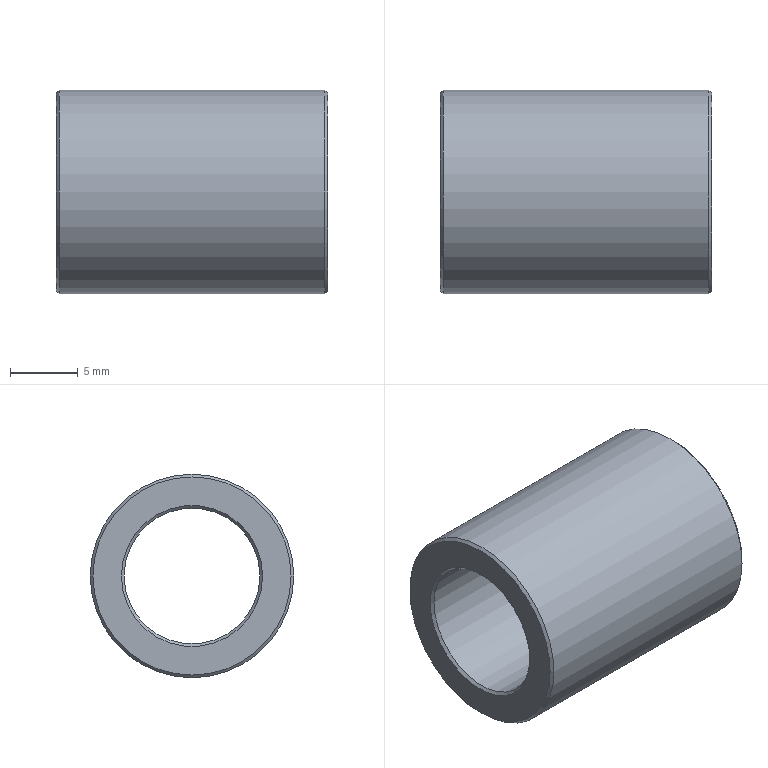Part | NX | features 5003_024_C-KNCLA10-15-20 2 | 1 solid | 8 faces | box 20 x 15 x 15 mm | volume 1960 mm3 | cone 4 | plane 2 | cylinder 2 | commonest cylinder face diameters 10 x1 15 x1
STEP:
#1=CARTESIAN_POINT('',(-233.475,-518.7,-147.));
#2=VERTEX_POINT('',#1);
#3=CARTESIAN_POINT('',(-233.475,-526.,-147.));
#4=DIRECTION('',(1.,0.,0.));
#5=DIRECTION('',(0.,1.,0.));
#6=AXIS2_PLACEMENT_3D('',#3,#4,#5);
#7=CIRCLE('',#6,7.3);
#8=EDGE_CURVE('',#2,#2,#7,.F.);
#9=ORIENTED_EDGE('',*,*,#8,.T.);
#10=EDGE_LOOP('',(#9));
#11=FACE_BOUND('',#10,.T.);
#12=CARTESIAN_POINT('',(-233.475,-520.8,-147.));
#13=VERTEX_POINT('',#12);
#14=CARTESIAN_POINT('',(-233.475,-526.,-147.));
#15=DIRECTION('',(1.,0.,0.));
#16=DIRECTION('',(0.,1.,0.));
#17=AXIS2_PLACEMENT_3D('',#14,#15,#16);
#18=CIRCLE('',#17,5.2);
#19=EDGE_CURVE('',#13,#13,#18,.T.);
#20=ORIENTED_EDGE('',*,*,#19,.T.);
#21=EDGE_LOOP('',(#20));
#22=FACE_BOUND('',#21,.T.);
#23=CARTESIAN_POINT('',(-233.475,-521.,-147.));
#24=DIRECTION('',(1.,0.,0.));
#25=DIRECTION('',(0.,1.,0.));
#26=AXIS2_PLACEMENT_3D('',#23,#24,#25);
#27=PLANE('',#26);
#28=ADVANCED_FACE('',(#11,#22),#27,.F.);
#29=CARTESIAN_POINT('',(-213.675,-533.5,-147.));
#30=VERTEX_POINT('',#29);
#31=CARTESIAN_POINT('',(-213.675,-526.,-147.));
#32=DIRECTION('',(-1.,0.,0.));
#33=DIRECTION('',(0.,-1.,0.));
#34=AXIS2_PLACEMENT_3D('',#31,#32,#33);
#35=CIRCLE('',#34,7.5);
#36=EDGE_CURVE('',#30,#30,#35,.T.);
#37=ORIENTED_EDGE('',*,*,#36,.T.);
#38=EDGE_LOOP('',(#37));
#39=FACE_BOUND('',#38,.T.);
#40=CARTESIAN_POINT('',(-233.275,-518.5,-147.));
#41=VERTEX_POINT('',#40);
#42=CARTESIAN_POINT('',(-233.275,-526.,-147.));
#43=DIRECTION('',(1.,0.,0.));
#44=DIRECTION('',(0.,1.,0.));
#45=AXIS2_PLACEMENT_3D('',#42,#43,#44);
#46=CIRCLE('',#45,7.5);
#47=EDGE_CURVE('',#41,#41,#46,.T.);
#48=ORIENTED_EDGE('',*,*,#47,.T.);
#49=EDGE_LOOP('',(#48));
#50=FACE_BOUND('',#49,.T.);
#51=CARTESIAN_POINT('',(-237.616,-526.,-147.));
#52=DIRECTION('',(-1.,0.,0.));
#53=DIRECTION('',(0.,-1.,0.));
#54=AXIS2_PLACEMENT_3D('',#51,#52,#53);
#55=CYLINDRICAL_SURFACE('',#54,7.5);
#56=ADVANCED_FACE('',(#39,#50),#55,.T.);
#57=CARTESIAN_POINT('',(-213.475,-533.3,-147.));
#58=VERTEX_POINT('',#57);
#59=CARTESIAN_POINT('',(-213.475,-526.,-147.));
#60=DIRECTION('',(-1.,0.,0.));
#61=DIRECTION('',(0.,-1.,0.));
#62=AXIS2_PLACEMENT_3D('',#59,#60,#61);
#63=CIRCLE('',#62,7.3);
#64=EDGE_CURVE('',#58,#58,#63,.F.);
#65=ORIENTED_EDGE('',*,*,#64,.T.);
#66=EDGE_LOOP('',(#65));
#67=FACE_BOUND('',#66,.T.);
#68=CARTESIAN_POINT('',(-213.475,-531.2,-147.));
#69=VERTEX_POINT('',#68);
#70=CARTESIAN_POINT('',(-213.475,-526.,-147.));
#71=DIRECTION('',(-1.,0.,0.));
#72=DIRECTION('',(0.,-1.,0.));
#73=AXIS2_PLACEMENT_3D('',#70,#71,#72);
#74=CIRCLE('',#73,5.2);
#75=EDGE_CURVE('',#69,#69,#74,.T.);
#76=ORIENTED_EDGE('',*,*,#75,.T.);
#77=EDGE_LOOP('',(#76));
#78=FACE_BOUND('',#77,.T.);
#79=CARTESIAN_POINT('',(-213.475,-521.,-147.));
#80=DIRECTION('',(-1.,0.,0.));
#81=DIRECTION('',(0.,-1.,0.));
#82=AXIS2_PLACEMENT_3D('',#79,#80,#81);
#83=PLANE('',#82);
#84=ADVANCED_FACE('',(#67,#78),#83,.F.);
#85=CARTESIAN_POINT('',(-213.675,-531.,-147.));
#86=VERTEX_POINT('',#85);
#87=CARTESIAN_POINT('',(-213.675,-526.,-147.));
#88=DIRECTION('',(-1.,0.,0.));
#89=DIRECTION('',(0.,-1.,0.));
#90=AXIS2_PLACEMENT_3D('',#87,#88,#89);
#91=CIRCLE('',#90,5.);
#92=EDGE_CURVE('',#86,#86,#91,.F.);
#93=ORIENTED_EDGE('',*,*,#92,.T.);
#94=EDGE_LOOP('',(#93));
#95=FACE_BOUND('',#94,.T.);
#96=CARTESIAN_POINT('',(-233.275,-521.,-147.));
#97=VERTEX_POINT('',#96);
#98=CARTESIAN_POINT('',(-233.275,-526.,-147.));
#99=DIRECTION('',(1.,0.,0.));
#100=DIRECTION('',(0.,1.,0.));
#101=AXIS2_PLACEMENT_3D('',#98,#99,#100);
#102=CIRCLE('',#101,5.);
#103=EDGE_CURVE('',#97,#97,#102,.F.);
#104=ORIENTED_EDGE('',*,*,#103,.T.);
#105=EDGE_LOOP('',(#104));
#106=FACE_BOUND('',#105,.T.);
#107=CARTESIAN_POINT('',(-237.616,-526.,-147.));
#108=DIRECTION('',(-1.,0.,0.));
#109=DIRECTION('',(0.,-1.,0.));
#110=AXIS2_PLACEMENT_3D('',#107,#108,#109);
#111=CYLINDRICAL_SURFACE('',#110,5.);
#112=ADVANCED_FACE('',(#95,#106),#111,.F.);
#113=ORIENTED_EDGE('',*,*,#64,.F.);
#114=EDGE_LOOP('',(#113));
#115=FACE_BOUND('',#114,.T.);
#116=ORIENTED_EDGE('',*,*,#36,.F.);
#117=EDGE_LOOP('',(#116));
#118=FACE_BOUND('',#117,.T.);
#119=CARTESIAN_POINT('',(-213.675,-526.,-147.));
#120=DIRECTION('',(-1.,0.,0.));
#121=DIRECTION('',(0.,-1.,0.));
#122=AXIS2_PLACEMENT_3D('',#119,#120,#121);
#123=CONICAL_SURFACE('',#122,7.5,0.7854);
#124=ADVANCED_FACE('',(#115,#118),#123,.T.);
#125=ORIENTED_EDGE('',*,*,#92,.F.);
#126=EDGE_LOOP('',(#125));
#127=FACE_BOUND('',#126,.T.);
#128=ORIENTED_EDGE('',*,*,#75,.F.);
#129=EDGE_LOOP('',(#128));
#130=FACE_BOUND('',#129,.T.);
#131=CARTESIAN_POINT('',(-213.475,-526.,-147.));
#132=DIRECTION('',(1.,0.,0.));
#133=DIRECTION('',(0.,1.,0.));
#134=AXIS2_PLACEMENT_3D('',#131,#132,#133);
#135=CONICAL_SURFACE('',#134,5.2,0.7854);
#136=ADVANCED_FACE('',(#127,#130),#135,.F.);
#137=ORIENTED_EDGE('',*,*,#47,.F.);
#138=EDGE_LOOP('',(#137));
#139=FACE_BOUND('',#138,.T.);
#140=ORIENTED_EDGE('',*,*,#8,.F.);
#141=EDGE_LOOP('',(#140));
#142=FACE_BOUND('',#141,.T.);
#143=CARTESIAN_POINT('',(-233.475,-526.,-147.));
#144=DIRECTION('',(1.,0.,0.));
#145=DIRECTION('',(0.,1.,0.));
#146=AXIS2_PLACEMENT_3D('',#143,#144,#145);
#147=CONICAL_SURFACE('',#146,7.3,0.7854);
#148=ADVANCED_FACE('',(#139,#142),#147,.T.);
#149=ORIENTED_EDGE('',*,*,#19,.F.);
#150=EDGE_LOOP('',(#149));
#151=FACE_BOUND('',#150,.T.);
#152=ORIENTED_EDGE('',*,*,#103,.F.);
#153=EDGE_LOOP('',(#152));
#154=FACE_BOUND('',#153,.T.);
#155=CARTESIAN_POINT('',(-233.275,-526.,-147.));
#156=DIRECTION('',(-1.,0.,0.));
#157=DIRECTION('',(0.,-1.,0.));
#158=AXIS2_PLACEMENT_3D('',#155,#156,#157);
#159=CONICAL_SURFACE('',#158,5.,0.7854);
#160=ADVANCED_FACE('',(#151,#154),#159,.F.);
#161=CLOSED_SHELL('',(#28,#56,#84,#112,#124,#136,#148,#160));
#162=MANIFOLD_SOLID_BREP('',#161);
#163=(LENGTH_UNIT()NAMED_UNIT(*)SI_UNIT(.MILLI.,.METRE.));
#164=UNCERTAINTY_MEASURE_WITH_UNIT(LENGTH_MEASURE(0.00001),#163,'','');
#165=(NAMED_UNIT(*)PLANE_ANGLE_UNIT()SI_UNIT($,.RADIAN.));
#166=(NAMED_UNIT(*)SI_UNIT($,.STERADIAN.)SOLID_ANGLE_UNIT());
#167=(GEOMETRIC_REPRESENTATION_CONTEXT(3)GLOBAL_UNCERTAINTY_ASSIGNED_CONTEXT((#164))GLOBAL_UNIT_ASSIGNED_CONTEXT((#163,#165,#166))REPRESENTATION_CONTEXT('',''));
#168=ADVANCED_BREP_SHAPE_REPRESENTATION('',(#162),#167);